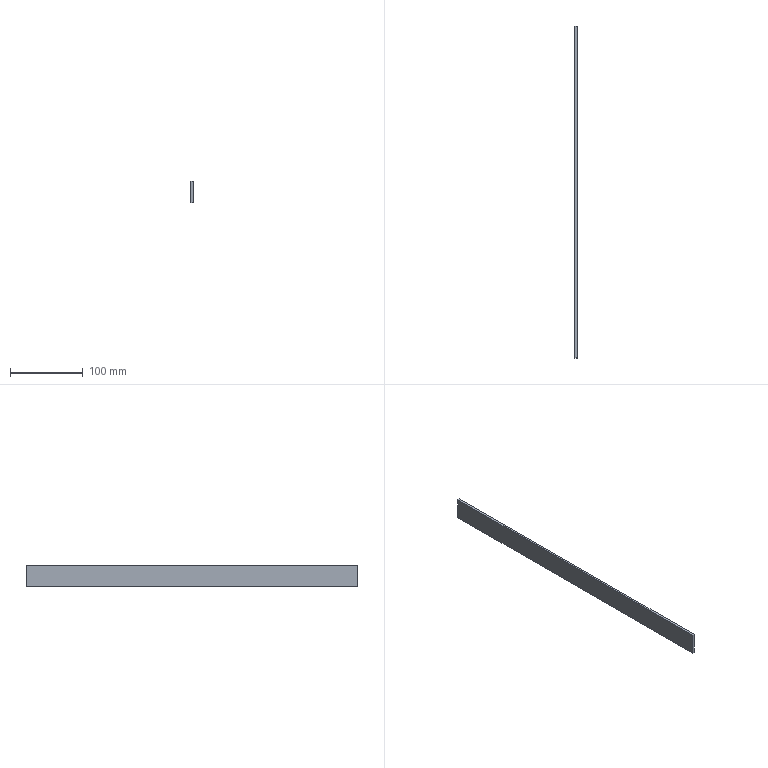Part | SolidWorks | 1 solid | 6 faces | box 3 x 455 x 30 mm | volume 40950 mm3 | plane 6
STEP:
#1=CARTESIAN_POINT('',(0.,227.5,15.));
#2=VERTEX_POINT('',#1);
#3=CARTESIAN_POINT('',(0.,-227.5,15.));
#4=VERTEX_POINT('',#3);
#5=CARTESIAN_POINT('',(0.,-227.5,15.));
#6=DIRECTION('',(0.,-1.,0.));
#7=VECTOR('',#6,1000.);
#8=LINE('',#5,#7);
#9=EDGE_CURVE('',#2,#4,#8,.T.);
#10=ORIENTED_EDGE('',*,*,#9,.F.);
#11=CARTESIAN_POINT('',(-3.,227.5,15.));
#12=VERTEX_POINT('',#11);
#13=CARTESIAN_POINT('',(-3.,227.5,15.));
#14=DIRECTION('',(1.,0.,0.));
#15=VECTOR('',#14,1000.);
#16=LINE('',#13,#15);
#17=EDGE_CURVE('',#12,#2,#16,.T.);
#18=ORIENTED_EDGE('',*,*,#17,.F.);
#19=CARTESIAN_POINT('',(-3.,-227.5,15.));
#20=VERTEX_POINT('',#19);
#21=CARTESIAN_POINT('',(-3.,-227.5,15.));
#22=DIRECTION('',(0.,-1.,0.));
#23=VECTOR('',#22,1000.);
#24=LINE('',#21,#23);
#25=EDGE_CURVE('',#12,#20,#24,.T.);
#26=ORIENTED_EDGE('',*,*,#25,.T.);
#27=CARTESIAN_POINT('',(-3.,-227.5,15.));
#28=DIRECTION('',(1.,0.,0.));
#29=VECTOR('',#28,1000.);
#30=LINE('',#27,#29);
#31=EDGE_CURVE('',#20,#4,#30,.T.);
#32=ORIENTED_EDGE('',*,*,#31,.T.);
#33=EDGE_LOOP('',(#10,#18,#26,#32));
#34=FACE_OUTER_BOUND('',#33,.T.);
#35=CARTESIAN_POINT('',(-3.,-227.5,15.));
#36=DIRECTION('',(0.,0.,1.));
#37=DIRECTION('',(1.,0.,0.));
#38=AXIS2_PLACEMENT_3D('',#35,#36,#37);
#39=PLANE('',#38);
#40=ADVANCED_FACE('',(#34),#39,.T.);
#41=CARTESIAN_POINT('',(0.,227.5,-15.));
#42=VERTEX_POINT('',#41);
#43=CARTESIAN_POINT('',(0.,227.5,-15.));
#44=DIRECTION('',(0.,0.,1.));
#45=VECTOR('',#44,1000.);
#46=LINE('',#43,#45);
#47=EDGE_CURVE('',#42,#2,#46,.T.);
#48=ORIENTED_EDGE('',*,*,#47,.F.);
#49=CARTESIAN_POINT('',(-3.,227.5,-15.));
#50=VERTEX_POINT('',#49);
#51=CARTESIAN_POINT('',(-3.,227.5,-15.));
#52=DIRECTION('',(1.,0.,0.));
#53=VECTOR('',#52,1000.);
#54=LINE('',#51,#53);
#55=EDGE_CURVE('',#50,#42,#54,.T.);
#56=ORIENTED_EDGE('',*,*,#55,.F.);
#57=CARTESIAN_POINT('',(-3.,227.5,-15.));
#58=DIRECTION('',(0.,0.,1.));
#59=VECTOR('',#58,1000.);
#60=LINE('',#57,#59);
#61=EDGE_CURVE('',#50,#12,#60,.T.);
#62=ORIENTED_EDGE('',*,*,#61,.T.);
#63=ORIENTED_EDGE('',*,*,#17,.T.);
#64=EDGE_LOOP('',(#48,#56,#62,#63));
#65=FACE_OUTER_BOUND('',#64,.T.);
#66=CARTESIAN_POINT('',(-3.,227.5,-15.));
#67=DIRECTION('',(0.,1.,0.));
#68=DIRECTION('',(0.,0.,1.));
#69=AXIS2_PLACEMENT_3D('',#66,#67,#68);
#70=PLANE('',#69);
#71=ADVANCED_FACE('',(#65),#70,.T.);
#72=CARTESIAN_POINT('',(0.,-227.5,-15.));
#73=VERTEX_POINT('',#72);
#74=CARTESIAN_POINT('',(0.,-227.5,-15.));
#75=DIRECTION('',(0.,1.,0.));
#76=VECTOR('',#75,1000.);
#77=LINE('',#74,#76);
#78=EDGE_CURVE('',#73,#42,#77,.T.);
#79=ORIENTED_EDGE('',*,*,#78,.F.);
#80=CARTESIAN_POINT('',(-3.,-227.5,-15.));
#81=VERTEX_POINT('',#80);
#82=CARTESIAN_POINT('',(-3.,-227.5,-15.));
#83=DIRECTION('',(1.,0.,0.));
#84=VECTOR('',#83,1000.);
#85=LINE('',#82,#84);
#86=EDGE_CURVE('',#81,#73,#85,.T.);
#87=ORIENTED_EDGE('',*,*,#86,.F.);
#88=CARTESIAN_POINT('',(-3.,-227.5,-15.));
#89=DIRECTION('',(0.,1.,0.));
#90=VECTOR('',#89,1000.);
#91=LINE('',#88,#90);
#92=EDGE_CURVE('',#81,#50,#91,.T.);
#93=ORIENTED_EDGE('',*,*,#92,.T.);
#94=ORIENTED_EDGE('',*,*,#55,.T.);
#95=EDGE_LOOP('',(#79,#87,#93,#94));
#96=FACE_OUTER_BOUND('',#95,.T.);
#97=CARTESIAN_POINT('',(-3.,-227.5,-15.));
#98=DIRECTION('',(0.,0.,-1.));
#99=DIRECTION('',(-1.,0.,0.));
#100=AXIS2_PLACEMENT_3D('',#97,#98,#99);
#101=PLANE('',#100);
#102=ADVANCED_FACE('',(#96),#101,.T.);
#103=CARTESIAN_POINT('',(0.,-227.5,-15.));
#104=DIRECTION('',(0.,0.,-1.));
#105=VECTOR('',#104,1000.);
#106=LINE('',#103,#105);
#107=EDGE_CURVE('',#4,#73,#106,.T.);
#108=ORIENTED_EDGE('',*,*,#107,.F.);
#109=ORIENTED_EDGE('',*,*,#31,.F.);
#110=CARTESIAN_POINT('',(-3.,-227.5,-15.));
#111=DIRECTION('',(0.,0.,-1.));
#112=VECTOR('',#111,1000.);
#113=LINE('',#110,#112);
#114=EDGE_CURVE('',#20,#81,#113,.T.);
#115=ORIENTED_EDGE('',*,*,#114,.T.);
#116=ORIENTED_EDGE('',*,*,#86,.T.);
#117=EDGE_LOOP('',(#108,#109,#115,#116));
#118=FACE_OUTER_BOUND('',#117,.T.);
#119=CARTESIAN_POINT('',(-3.,-227.5,-15.));
#120=DIRECTION('',(0.,-1.,0.));
#121=DIRECTION('',(0.,0.,-1.));
#122=AXIS2_PLACEMENT_3D('',#119,#120,#121);
#123=PLANE('',#122);
#124=ADVANCED_FACE('',(#118),#123,.T.);
#125=ORIENTED_EDGE('',*,*,#25,.F.);
#126=ORIENTED_EDGE('',*,*,#61,.F.);
#127=ORIENTED_EDGE('',*,*,#92,.F.);
#128=ORIENTED_EDGE('',*,*,#114,.F.);
#129=EDGE_LOOP('',(#125,#126,#127,#128));
#130=FACE_OUTER_BOUND('',#129,.T.);
#131=CARTESIAN_POINT('',(-3.,0.,0.));
#132=DIRECTION('',(1.,0.,0.));
#133=DIRECTION('',(0.,0.,-1.));
#134=AXIS2_PLACEMENT_3D('',#131,#132,#133);
#135=PLANE('',#134);
#136=ADVANCED_FACE('',(#130),#135,.F.);
#137=ORIENTED_EDGE('',*,*,#9,.T.);
#138=ORIENTED_EDGE('',*,*,#107,.T.);
#139=ORIENTED_EDGE('',*,*,#78,.T.);
#140=ORIENTED_EDGE('',*,*,#47,.T.);
#141=EDGE_LOOP('',(#137,#138,#139,#140));
#142=FACE_OUTER_BOUND('',#141,.T.);
#143=CARTESIAN_POINT('',(0.,0.,0.));
#144=DIRECTION('',(1.,0.,0.));
#145=DIRECTION('',(0.,0.,-1.));
#146=AXIS2_PLACEMENT_3D('',#143,#144,#145);
#147=PLANE('',#146);
#148=ADVANCED_FACE('',(#142),#147,.T.);
#149=CLOSED_SHELL('',(#40,#71,#102,#124,#136,#148));
#150=MANIFOLD_SOLID_BREP('',#149);
#151=CARTESIAN_POINT('',(0.,0.,0.));
#152=DIRECTION('',(0.,0.,1.));
#153=DIRECTION('',(1.,0.,0.));
#154=AXIS2_PLACEMENT_3D('',#151,#152,#153);
#155=(LENGTH_UNIT()NAMED_UNIT(*)SI_UNIT(.MILLI.,.METRE.));
#156=UNCERTAINTY_MEASURE_WITH_UNIT(LENGTH_MEASURE(0.00001),#155,'','');
#157=(NAMED_UNIT(*)PLANE_ANGLE_UNIT()SI_UNIT($,.RADIAN.));
#158=(NAMED_UNIT(*)SI_UNIT($,.STERADIAN.)SOLID_ANGLE_UNIT());
#159=(GEOMETRIC_REPRESENTATION_CONTEXT(3)GLOBAL_UNCERTAINTY_ASSIGNED_CONTEXT((#156))GLOBAL_UNIT_ASSIGNED_CONTEXT((#155,#157,#158))REPRESENTATION_CONTEXT('',''));
#160=ADVANCED_BREP_SHAPE_REPRESENTATION('',(#150,#154),#159);